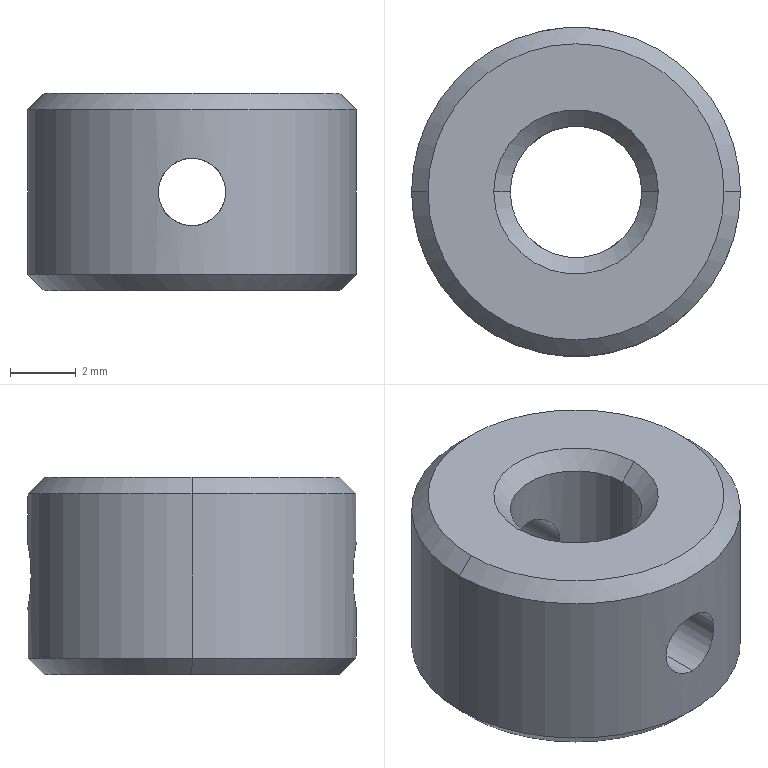Part | SolidWorks | features BaseBody 1, Chamfer 1 | 1 solid | 18 faces | box 10 x 10 x 6 mm | volume 364.767 mm3 | cone 8 | cylinder 8 | plane 2 | commonest cylinder face diameters 2.05 x4 4 x2 10 x2
STEP:
#1=CARTESIAN_POINT('',(-4.5,0.,-3.));
#2=VERTEX_POINT('',#1);
#3=CARTESIAN_POINT('',(4.5,0.,-3.));
#4=VERTEX_POINT('',#3);
#5=CARTESIAN_POINT('',(0.,0.,-3.));
#6=DIRECTION('',(0.,0.,-1.));
#7=DIRECTION('',(1.,0.,0.));
#8=AXIS2_PLACEMENT_3D('',#5,#6,#7);
#9=CIRCLE('',#8,4.5);
#10=EDGE_CURVE('',#2,#4,#9,.T.);
#11=ORIENTED_EDGE('',*,*,#10,.F.);
#12=CARTESIAN_POINT('',(-5.,0.,-2.5));
#13=VERTEX_POINT('',#12);
#14=CARTESIAN_POINT('',(-5.,0.,-2.5));
#15=DIRECTION('',(-0.7071,0.,0.7071));
#16=VECTOR('',#15,1000.);
#17=LINE('',#14,#16);
#18=EDGE_CURVE('',#2,#13,#17,.T.);
#19=ORIENTED_EDGE('',*,*,#18,.T.);
#20=CARTESIAN_POINT('',(5.,0.,-2.5));
#21=VERTEX_POINT('',#20);
#22=CARTESIAN_POINT('',(0.,0.,-2.5));
#23=DIRECTION('',(0.,0.,1.));
#24=DIRECTION('',(1.,0.,0.));
#25=AXIS2_PLACEMENT_3D('',#22,#23,#24);
#26=CIRCLE('',#25,5.);
#27=EDGE_CURVE('',#21,#13,#26,.T.);
#28=ORIENTED_EDGE('',*,*,#27,.F.);
#29=CARTESIAN_POINT('',(5.,0.,-2.5));
#30=DIRECTION('',(0.7071,0.,0.7071));
#31=VECTOR('',#30,1000.);
#32=LINE('',#29,#31);
#33=EDGE_CURVE('',#4,#21,#32,.T.);
#34=ORIENTED_EDGE('',*,*,#33,.F.);
#35=EDGE_LOOP('',(#11,#19,#28,#34));
#36=FACE_OUTER_BOUND('',#35,.T.);
#37=CARTESIAN_POINT('',(0.,0.,-2.5));
#38=DIRECTION('',(0.,0.,1.));
#39=DIRECTION('',(1.,0.,0.));
#40=AXIS2_PLACEMENT_3D('',#37,#38,#39);
#41=CONICAL_SURFACE('',#40,5.,0.7854);
#42=ADVANCED_FACE('',(#36),#41,.T.);
#43=CARTESIAN_POINT('',(4.5,0.,3.));
#44=VERTEX_POINT('',#43);
#45=CARTESIAN_POINT('',(-4.5,0.,3.));
#46=VERTEX_POINT('',#45);
#47=CARTESIAN_POINT('',(0.,0.,3.));
#48=DIRECTION('',(0.,0.,1.));
#49=DIRECTION('',(1.,0.,0.));
#50=AXIS2_PLACEMENT_3D('',#47,#48,#49);
#51=CIRCLE('',#50,4.5);
#52=EDGE_CURVE('',#44,#46,#51,.T.);
#53=ORIENTED_EDGE('',*,*,#52,.F.);
#54=CARTESIAN_POINT('',(5.,0.,2.5));
#55=VERTEX_POINT('',#54);
#56=CARTESIAN_POINT('',(5.,0.,2.5));
#57=DIRECTION('',(0.7071,0.,-0.7071));
#58=VECTOR('',#57,1000.);
#59=LINE('',#56,#58);
#60=EDGE_CURVE('',#44,#55,#59,.T.);
#61=ORIENTED_EDGE('',*,*,#60,.T.);
#62=CARTESIAN_POINT('',(-5.,0.,2.5));
#63=VERTEX_POINT('',#62);
#64=CARTESIAN_POINT('',(0.,0.,2.5));
#65=DIRECTION('',(0.,0.,-1.));
#66=DIRECTION('',(1.,0.,0.));
#67=AXIS2_PLACEMENT_3D('',#64,#65,#66);
#68=CIRCLE('',#67,5.);
#69=EDGE_CURVE('',#63,#55,#68,.T.);
#70=ORIENTED_EDGE('',*,*,#69,.F.);
#71=CARTESIAN_POINT('',(-5.,0.,2.5));
#72=DIRECTION('',(-0.7071,0.,-0.7071));
#73=VECTOR('',#72,1000.);
#74=LINE('',#71,#73);
#75=EDGE_CURVE('',#46,#63,#74,.T.);
#76=ORIENTED_EDGE('',*,*,#75,.F.);
#77=EDGE_LOOP('',(#53,#61,#70,#76));
#78=FACE_OUTER_BOUND('',#77,.T.);
#79=CARTESIAN_POINT('',(0.,0.,2.5));
#80=DIRECTION('',(0.,0.,-1.));
#81=DIRECTION('',(-1.,0.,0.));
#82=AXIS2_PLACEMENT_3D('',#79,#80,#81);
#83=CONICAL_SURFACE('',#82,5.,0.7854);
#84=ADVANCED_FACE('',(#78),#83,.T.);
#85=CARTESIAN_POINT('',(-2.,0.,2.5));
#86=VERTEX_POINT('',#85);
#87=CARTESIAN_POINT('',(2.,0.,2.5));
#88=VERTEX_POINT('',#87);
#89=CARTESIAN_POINT('',(0.,0.,2.5));
#90=DIRECTION('',(0.,0.,1.));
#91=DIRECTION('',(1.,0.,0.));
#92=AXIS2_PLACEMENT_3D('',#89,#90,#91);
#93=CIRCLE('',#92,2.);
#94=EDGE_CURVE('',#86,#88,#93,.T.);
#95=ORIENTED_EDGE('',*,*,#94,.F.);
#96=CARTESIAN_POINT('',(-2.5,0.,3.));
#97=VERTEX_POINT('',#96);
#98=CARTESIAN_POINT('',(-2.5,0.,3.));
#99=DIRECTION('',(-0.7071,0.,0.7071));
#100=VECTOR('',#99,1000.);
#101=LINE('',#98,#100);
#102=EDGE_CURVE('',#86,#97,#101,.T.);
#103=ORIENTED_EDGE('',*,*,#102,.T.);
#104=CARTESIAN_POINT('',(2.5,0.,3.));
#105=VERTEX_POINT('',#104);
#106=CARTESIAN_POINT('',(0.,0.,3.));
#107=DIRECTION('',(0.,0.,-1.));
#108=DIRECTION('',(1.,0.,0.));
#109=AXIS2_PLACEMENT_3D('',#106,#107,#108);
#110=CIRCLE('',#109,2.5);
#111=EDGE_CURVE('',#105,#97,#110,.T.);
#112=ORIENTED_EDGE('',*,*,#111,.F.);
#113=CARTESIAN_POINT('',(2.5,0.,3.));
#114=DIRECTION('',(0.7071,0.,0.7071));
#115=VECTOR('',#114,1000.);
#116=LINE('',#113,#115);
#117=EDGE_CURVE('',#88,#105,#116,.T.);
#118=ORIENTED_EDGE('',*,*,#117,.F.);
#119=EDGE_LOOP('',(#95,#103,#112,#118));
#120=FACE_OUTER_BOUND('',#119,.T.);
#121=CARTESIAN_POINT('',(0.,0.,3.));
#122=DIRECTION('',(0.,0.,1.));
#123=DIRECTION('',(1.,0.,0.));
#124=AXIS2_PLACEMENT_3D('',#121,#122,#123);
#125=CONICAL_SURFACE('',#124,2.5,0.7854);
#126=ADVANCED_FACE('',(#120),#125,.F.);
#127=CARTESIAN_POINT('',(2.,0.,-2.5));
#128=VERTEX_POINT('',#127);
#129=CARTESIAN_POINT('',(-2.,0.,-2.5));
#130=VERTEX_POINT('',#129);
#131=CARTESIAN_POINT('',(0.,0.,-2.5));
#132=DIRECTION('',(0.,0.,-1.));
#133=DIRECTION('',(1.,0.,0.));
#134=AXIS2_PLACEMENT_3D('',#131,#132,#133);
#135=CIRCLE('',#134,2.);
#136=EDGE_CURVE('',#128,#130,#135,.T.);
#137=ORIENTED_EDGE('',*,*,#136,.F.);
#138=CARTESIAN_POINT('',(2.5,0.,-3.));
#139=VERTEX_POINT('',#138);
#140=CARTESIAN_POINT('',(2.,0.,-2.5));
#141=DIRECTION('',(0.7071,0.,-0.7071));
#142=VECTOR('',#141,1000.);
#143=LINE('',#140,#142);
#144=EDGE_CURVE('',#128,#139,#143,.T.);
#145=ORIENTED_EDGE('',*,*,#144,.T.);
#146=CARTESIAN_POINT('',(-2.5,0.,-3.));
#147=VERTEX_POINT('',#146);
#148=CARTESIAN_POINT('',(0.,0.,-3.));
#149=DIRECTION('',(0.,0.,1.));
#150=DIRECTION('',(1.,0.,0.));
#151=AXIS2_PLACEMENT_3D('',#148,#149,#150);
#152=CIRCLE('',#151,2.5);
#153=EDGE_CURVE('',#147,#139,#152,.T.);
#154=ORIENTED_EDGE('',*,*,#153,.F.);
#155=CARTESIAN_POINT('',(-2.,0.,-2.5));
#156=DIRECTION('',(-0.7071,0.,-0.7071));
#157=VECTOR('',#156,1000.);
#158=LINE('',#155,#157);
#159=EDGE_CURVE('',#130,#147,#158,.T.);
#160=ORIENTED_EDGE('',*,*,#159,.F.);
#161=EDGE_LOOP('',(#137,#145,#154,#160));
#162=FACE_OUTER_BOUND('',#161,.T.);
#163=CARTESIAN_POINT('',(0.,0.,-2.5));
#164=DIRECTION('',(0.,0.,-1.));
#165=DIRECTION('',(-1.,0.,0.));
#166=AXIS2_PLACEMENT_3D('',#163,#164,#165);
#167=CONICAL_SURFACE('',#166,2.,0.7854);
#168=ADVANCED_FACE('',(#162),#167,.F.);
#169=CARTESIAN_POINT('',(0.,5.,-1.025));
#170=VERTEX_POINT('',#169);
#171=CARTESIAN_POINT('',(0.,5.,1.025));
#172=VERTEX_POINT('',#171);
#173=CARTESIAN_POINT('',(0.,5.,-1.025));
#174=CARTESIAN_POINT('',(0.1358,5.,-1.025));
#175=CARTESIAN_POINT('',(0.269,4.994,-0.9981));
#176=CARTESIAN_POINT('',(0.5171,4.975,-0.8951));
#177=CARTESIAN_POINT('',(0.6306,4.961,-0.819));
#178=CARTESIAN_POINT('',(0.8191,4.933,-0.6305));
#179=CARTESIAN_POINT('',(0.8954,4.919,-0.5165));
#180=CARTESIAN_POINT('',(0.9978,4.9,-0.27));
#181=CARTESIAN_POINT('',(1.025,4.894,-0.1349));
#182=CARTESIAN_POINT('',(1.025,4.894,0.1332));
#183=CARTESIAN_POINT('',(0.9985,4.9,0.2677));
#184=CARTESIAN_POINT('',(0.8956,4.919,0.5163));
#185=CARTESIAN_POINT('',(0.8204,4.933,0.6291));
#186=CARTESIAN_POINT('',(0.63,4.961,0.8197));
#187=CARTESIAN_POINT('',(0.5172,4.975,0.895));
#188=CARTESIAN_POINT('',(0.2695,4.994,0.998));
#189=CARTESIAN_POINT('',(0.1358,5.,1.025));
#190=CARTESIAN_POINT('',(0.,5.,1.025));
#191=B_SPLINE_CURVE_WITH_KNOTS('',3,(#173,#174,#175,#176,#177,#178,#179,#180,#181,#182,#183,#184,#185,#186,#187,#188,#189,#190),.UNSPECIFIED.,.F.,.F.,(4,2,2,2,2,2,2,2,4),(0.,0.0004015,0.0008031,0.001205,0.001606,0.002008,0.002409,0.002811,0.003212),.UNSPECIFIED.);
#192=EDGE_CURVE('',#170,#172,#191,.T.);
#193=ORIENTED_EDGE('',*,*,#192,.T.);
#194=CARTESIAN_POINT('',(0.,5.,1.025));
#195=CARTESIAN_POINT('',(-0.1358,5.,1.025));
#196=CARTESIAN_POINT('',(-0.269,4.994,0.9981));
#197=CARTESIAN_POINT('',(-0.5171,4.975,0.8951));
#198=CARTESIAN_POINT('',(-0.6306,4.961,0.819));
#199=CARTESIAN_POINT('',(-0.8191,4.933,0.6305));
#200=CARTESIAN_POINT('',(-0.8954,4.919,0.5165));
#201=CARTESIAN_POINT('',(-0.9978,4.9,0.27));
#202=CARTESIAN_POINT('',(-1.025,4.894,0.1349));
#203=CARTESIAN_POINT('',(-1.025,4.894,-0.1332));
#204=CARTESIAN_POINT('',(-0.9985,4.9,-0.2677));
#205=CARTESIAN_POINT('',(-0.8956,4.919,-0.5163));
#206=CARTESIAN_POINT('',(-0.8204,4.933,-0.6291));
#207=CARTESIAN_POINT('',(-0.63,4.961,-0.8197));
#208=CARTESIAN_POINT('',(-0.5172,4.975,-0.895));
#209=CARTESIAN_POINT('',(-0.2695,4.994,-0.998));
#210=CARTESIAN_POINT('',(-0.1358,5.,-1.025));
#211=CARTESIAN_POINT('',(0.,5.,-1.025));
#212=B_SPLINE_CURVE_WITH_KNOTS('',3,(#194,#195,#196,#197,#198,#199,#200,#201,#202,#203,#204,#205,#206,#207,#208,#209,#210,#211),.UNSPECIFIED.,.F.,.F.,(4,2,2,2,2,2,2,2,4),(0.003212,0.003614,0.004015,0.004417,0.004818,0.00522,0.005621,0.006023,0.006425),.UNSPECIFIED.);
#213=EDGE_CURVE('',#172,#170,#212,.T.);
#214=ORIENTED_EDGE('',*,*,#213,.T.);
#215=EDGE_LOOP('',(#193,#214));
#216=FACE_BOUND('',#215,.T.);
#217=ORIENTED_EDGE('',*,*,#69,.T.);
#218=CARTESIAN_POINT('',(5.,0.,3.));
#219=DIRECTION('',(0.,0.,-1.));
#220=VECTOR('',#219,1000.);
#221=LINE('',#218,#220);
#222=EDGE_CURVE('',#55,#21,#221,.T.);
#223=ORIENTED_EDGE('',*,*,#222,.T.);
#224=ORIENTED_EDGE('',*,*,#27,.T.);
#225=CARTESIAN_POINT('',(-5.,0.,3.));
#226=DIRECTION('',(0.,0.,-1.));
#227=VECTOR('',#226,1000.);
#228=LINE('',#225,#227);
#229=EDGE_CURVE('',#63,#13,#228,.T.);
#230=ORIENTED_EDGE('',*,*,#229,.F.);
#231=EDGE_LOOP('',(#217,#223,#224,#230));
#232=FACE_OUTER_BOUND('',#231,.T.);
#233=CARTESIAN_POINT('',(0.,0.,3.));
#234=DIRECTION('',(0.,0.,-1.));
#235=DIRECTION('',(-1.,0.,0.));
#236=AXIS2_PLACEMENT_3D('',#233,#234,#235);
#237=CYLINDRICAL_SURFACE('',#236,5.);
#238=ADVANCED_FACE('',(#216,#232),#237,.T.);
#239=ORIENTED_EDGE('',*,*,#213,.F.);
#240=CARTESIAN_POINT('',(0.,2.,1.025));
#241=VERTEX_POINT('',#240);
#242=CARTESIAN_POINT('',(0.,0.,1.025));
#243=DIRECTION('',(0.,-1.,0.));
#244=VECTOR('',#243,1000.);
#245=LINE('',#242,#244);
#246=EDGE_CURVE('',#172,#241,#245,.T.);
#247=ORIENTED_EDGE('',*,*,#246,.T.);
#248=CARTESIAN_POINT('',(0.,2.,-1.025));
#249=VERTEX_POINT('',#248);
#250=CARTESIAN_POINT('',(0.,2.,-1.025));
#251=CARTESIAN_POINT('',(-0.138,2.,-1.025));
#252=CARTESIAN_POINT('',(-0.2732,1.985,-0.997));
#253=CARTESIAN_POINT('',(-0.5207,1.935,-0.893));
#254=CARTESIAN_POINT('',(-0.6326,1.9,-0.8171));
#255=CARTESIAN_POINT('',(-0.8181,1.828,-0.6313));
#256=CARTESIAN_POINT('',(-0.8935,1.79,-0.5197));
#257=CARTESIAN_POINT('',(-0.9965,1.735,-0.2744));
#258=CARTESIAN_POINT('',(-1.025,1.718,-0.1384));
#259=CARTESIAN_POINT('',(-1.025,1.717,0.1346));
#260=CARTESIAN_POINT('',(-0.9975,1.734,0.2713));
#261=CARTESIAN_POINT('',(-0.8938,1.79,0.5194));
#262=CARTESIAN_POINT('',(-0.8185,1.828,0.6308));
#263=CARTESIAN_POINT('',(-0.633,1.9,0.8168));
#264=CARTESIAN_POINT('',(-0.5207,1.935,0.8929));
#265=CARTESIAN_POINT('',(-0.2749,1.985,0.9964));
#266=CARTESIAN_POINT('',(-0.1382,2.,1.025));
#267=CARTESIAN_POINT('',(0.,2.,1.025));
#268=B_SPLINE_CURVE_WITH_KNOTS('',3,(#250,#251,#252,#253,#254,#255,#256,#257,#258,#259,#260,#261,#262,#263,#264,#265,#266,#267),.UNSPECIFIED.,.F.,.F.,(4,2,2,2,2,2,2,2,4),(0.,0.0004078,0.0008155,0.001223,0.001631,0.002039,0.002447,0.002854,0.003262),.UNSPECIFIED.);
#269=EDGE_CURVE('',#249,#241,#268,.T.);
#270=ORIENTED_EDGE('',*,*,#269,.F.);
#271=CARTESIAN_POINT('',(0.,0.,-1.025));
#272=DIRECTION('',(0.,-1.,0.));
#273=VECTOR('',#272,1000.);
#274=LINE('',#271,#273);
#275=EDGE_CURVE('',#170,#249,#274,.T.);
#276=ORIENTED_EDGE('',*,*,#275,.F.);
#277=EDGE_LOOP('',(#239,#247,#270,#276));
#278=FACE_OUTER_BOUND('',#277,.T.);
#279=CARTESIAN_POINT('',(0.,0.,0.));
#280=DIRECTION('',(0.,-1.,0.));
#281=DIRECTION('',(0.,0.,-1.));
#282=AXIS2_PLACEMENT_3D('',#279,#280,#281);
#283=CYLINDRICAL_SURFACE('',#282,1.025);
#284=ADVANCED_FACE('',(#278),#283,.F.);
#285=CARTESIAN_POINT('',(0.,-5.,-1.025));
#286=VERTEX_POINT('',#285);
#287=CARTESIAN_POINT('',(0.,-5.,1.025));
#288=VERTEX_POINT('',#287);
#289=CARTESIAN_POINT('',(0.,-5.,-1.025));
#290=CARTESIAN_POINT('',(-0.1358,-5.,-1.025));
#291=CARTESIAN_POINT('',(-0.269,-4.994,-0.9981));
#292=CARTESIAN_POINT('',(-0.5171,-4.975,-0.8951));
#293=CARTESIAN_POINT('',(-0.6306,-4.961,-0.819));
#294=CARTESIAN_POINT('',(-0.8191,-4.933,-0.6305));
#295=CARTESIAN_POINT('',(-0.8954,-4.919,-0.5165));
#296=CARTESIAN_POINT('',(-0.9978,-4.9,-0.27));
#297=CARTESIAN_POINT('',(-1.025,-4.894,-0.1349));
#298=CARTESIAN_POINT('',(-1.025,-4.894,0.1332));
#299=CARTESIAN_POINT('',(-0.9985,-4.9,0.2677));
#300=CARTESIAN_POINT('',(-0.8956,-4.919,0.5163));
#301=CARTESIAN_POINT('',(-0.8204,-4.933,0.6291));
#302=CARTESIAN_POINT('',(-0.63,-4.961,0.8197));
#303=CARTESIAN_POINT('',(-0.5172,-4.975,0.895));
#304=CARTESIAN_POINT('',(-0.2695,-4.994,0.998));
#305=CARTESIAN_POINT('',(-0.1358,-5.,1.025));
#306=CARTESIAN_POINT('',(0.,-5.,1.025));
#307=B_SPLINE_CURVE_WITH_KNOTS('',3,(#289,#290,#291,#292,#293,#294,#295,#296,#297,#298,#299,#300,#301,#302,#303,#304,#305,#306),.UNSPECIFIED.,.F.,.F.,(4,2,2,2,2,2,2,2,4),(0.,0.0004015,0.0008031,0.001205,0.001606,0.002008,0.002409,0.002811,0.003212),.UNSPECIFIED.);
#308=EDGE_CURVE('',#286,#288,#307,.T.);
#309=ORIENTED_EDGE('',*,*,#308,.F.);
#310=CARTESIAN_POINT('',(0.,-2.,-1.025));
#311=VERTEX_POINT('',#310);
#312=CARTESIAN_POINT('',(0.,0.,-1.025));
#313=DIRECTION('',(0.,1.,0.));
#314=VECTOR('',#313,1000.);
#315=LINE('',#312,#314);
#316=EDGE_CURVE('',#286,#311,#315,.T.);
#317=ORIENTED_EDGE('',*,*,#316,.T.);
#318=CARTESIAN_POINT('',(0.,-2.,1.025));
#319=VERTEX_POINT('',#318);
#320=CARTESIAN_POINT('',(0.,-2.,1.025));
#321=CARTESIAN_POINT('',(-0.138,-2.,1.025));
#322=CARTESIAN_POINT('',(-0.2732,-1.985,0.997));
#323=CARTESIAN_POINT('',(-0.5207,-1.935,0.893));
#324=CARTESIAN_POINT('',(-0.6326,-1.9,0.8171));
#325=CARTESIAN_POINT('',(-0.8181,-1.828,0.6313));
#326=CARTESIAN_POINT('',(-0.8935,-1.79,0.5197));
#327=CARTESIAN_POINT('',(-0.9965,-1.735,0.2744));
#328=CARTESIAN_POINT('',(-1.025,-1.718,0.1384));
#329=CARTESIAN_POINT('',(-1.025,-1.717,-0.1346));
#330=CARTESIAN_POINT('',(-0.9975,-1.734,-0.2713));
#331=CARTESIAN_POINT('',(-0.8938,-1.79,-0.5194));
#332=CARTESIAN_POINT('',(-0.8185,-1.828,-0.6308));
#333=CARTESIAN_POINT('',(-0.633,-1.9,-0.8168));
#334=CARTESIAN_POINT('',(-0.5207,-1.935,-0.8929));
#335=CARTESIAN_POINT('',(-0.2749,-1.985,-0.9964));
#336=CARTESIAN_POINT('',(-0.1382,-2.,-1.025));
#337=CARTESIAN_POINT('',(0.,-2.,-1.025));
#338=B_SPLINE_CURVE_WITH_KNOTS('',3,(#320,#321,#322,#323,#324,#325,#326,#327,#328,#329,#330,#331,#332,#333,#334,#335,#336,#337),.UNSPECIFIED.,.F.,.F.,(4,2,2,2,2,2,2,2,4),(0.,0.0004078,0.0008155,0.001223,0.001631,0.002039,0.002447,0.002854,0.003262),.UNSPECIFIED.);
#339=EDGE_CURVE('',#319,#311,#338,.T.);
#340=ORIENTED_EDGE('',*,*,#339,.F.);
#341=CARTESIAN_POINT('',(0.,0.,1.025));
#342=DIRECTION('',(0.,1.,0.));
#343=VECTOR('',#342,1000.);
#344=LINE('',#341,#343);
#345=EDGE_CURVE('',#288,#319,#344,.T.);
#346=ORIENTED_EDGE('',*,*,#345,.F.);
#347=EDGE_LOOP('',(#309,#317,#340,#346));
#348=FACE_OUTER_BOUND('',#347,.T.);
#349=CARTESIAN_POINT('',(0.,0.,0.));
#350=DIRECTION('',(0.,1.,0.));
#351=DIRECTION('',(0.,0.,1.));
#352=AXIS2_PLACEMENT_3D('',#349,#350,#351);
#353=CYLINDRICAL_SURFACE('',#352,1.025);
#354=ADVANCED_FACE('',(#348),#353,.F.);
#355=ORIENTED_EDGE('',*,*,#339,.T.);
#356=CARTESIAN_POINT('',(0.,-2.,-1.025));
#357=CARTESIAN_POINT('',(0.138,-2.,-1.025));
#358=CARTESIAN_POINT('',(0.2732,-1.985,-0.997));
#359=CARTESIAN_POINT('',(0.5207,-1.935,-0.893));
#360=CARTESIAN_POINT('',(0.6326,-1.9,-0.8171));
#361=CARTESIAN_POINT('',(0.8181,-1.828,-0.6313));
#362=CARTESIAN_POINT('',(0.8935,-1.79,-0.5197));
#363=CARTESIAN_POINT('',(0.9965,-1.735,-0.2744));
#364=CARTESIAN_POINT('',(1.025,-1.718,-0.1384));
#365=CARTESIAN_POINT('',(1.025,-1.717,0.1346));
#366=CARTESIAN_POINT('',(0.9975,-1.734,0.2713));
#367=CARTESIAN_POINT('',(0.8938,-1.79,0.5194));
#368=CARTESIAN_POINT('',(0.8185,-1.828,0.6308));
#369=CARTESIAN_POINT('',(0.633,-1.9,0.8168));
#370=CARTESIAN_POINT('',(0.5207,-1.935,0.8929));
#371=CARTESIAN_POINT('',(0.2749,-1.985,0.9964));
#372=CARTESIAN_POINT('',(0.1379,-2.,1.025));
#373=CARTESIAN_POINT('',(0.,-2.,1.025));
#374=B_SPLINE_CURVE_WITH_KNOTS('',3,(#356,#357,#358,#359,#360,#361,#362,#363,#364,#365,#366,#367,#368,#369,#370,#371,#372,#373),.UNSPECIFIED.,.F.,.F.,(4,2,2,2,2,2,2,2,4),(0.003262,0.003669,0.004077,0.004484,0.004891,0.005299,0.005706,0.006114,0.006521),.UNSPECIFIED.);
#375=EDGE_CURVE('',#311,#319,#374,.T.);
#376=ORIENTED_EDGE('',*,*,#375,.T.);
#377=EDGE_LOOP('',(#355,#376));
#378=FACE_BOUND('',#377,.T.);
#379=ORIENTED_EDGE('',*,*,#94,.T.);
#380=CARTESIAN_POINT('',(2.,0.,3.));
#381=DIRECTION('',(0.,0.,-1.));
#382=VECTOR('',#381,1000.);
#383=LINE('',#380,#382);
#384=EDGE_CURVE('',#88,#128,#383,.T.);
#385=ORIENTED_EDGE('',*,*,#384,.T.);
#386=ORIENTED_EDGE('',*,*,#136,.T.);
#387=CARTESIAN_POINT('',(-2.,0.,3.));
#388=DIRECTION('',(0.,0.,-1.));
#389=VECTOR('',#388,1000.);
#390=LINE('',#387,#389);
#391=EDGE_CURVE('',#86,#130,#390,.T.);
#392=ORIENTED_EDGE('',*,*,#391,.F.);
#393=EDGE_LOOP('',(#379,#385,#386,#392));
#394=FACE_OUTER_BOUND('',#393,.T.);
#395=CARTESIAN_POINT('',(0.,0.,3.));
#396=DIRECTION('',(0.,0.,-1.));
#397=DIRECTION('',(-1.,0.,0.));
#398=AXIS2_PLACEMENT_3D('',#395,#396,#397);
#399=CYLINDRICAL_SURFACE('',#398,2.);
#400=ADVANCED_FACE('',(#378,#394),#399,.F.);
#401=ORIENTED_EDGE('',*,*,#222,.F.);
#402=CARTESIAN_POINT('',(0.,0.,2.5));
#403=DIRECTION('',(0.,0.,-1.));
#404=DIRECTION('',(1.,0.,0.));
#405=AXIS2_PLACEMENT_3D('',#402,#403,#404);
#406=CIRCLE('',#405,5.);
#407=EDGE_CURVE('',#55,#63,#406,.T.);
#408=ORIENTED_EDGE('',*,*,#407,.T.);
#409=ORIENTED_EDGE('',*,*,#229,.T.);
#410=CARTESIAN_POINT('',(0.,0.,-2.5));
#411=DIRECTION('',(0.,0.,1.));
#412=DIRECTION('',(1.,0.,0.));
#413=AXIS2_PLACEMENT_3D('',#410,#411,#412);
#414=CIRCLE('',#413,5.);
#415=EDGE_CURVE('',#13,#21,#414,.T.);
#416=ORIENTED_EDGE('',*,*,#415,.T.);
#417=EDGE_LOOP('',(#401,#408,#409,#416));
#418=FACE_OUTER_BOUND('',#417,.T.);
#419=CARTESIAN_POINT('',(0.,-5.,1.025));
#420=CARTESIAN_POINT('',(0.1358,-5.,1.025));
#421=CARTESIAN_POINT('',(0.269,-4.994,0.9981));
#422=CARTESIAN_POINT('',(0.5171,-4.975,0.8951));
#423=CARTESIAN_POINT('',(0.6306,-4.961,0.819));
#424=CARTESIAN_POINT('',(0.8191,-4.933,0.6305));
#425=CARTESIAN_POINT('',(0.8954,-4.919,0.5165));
#426=CARTESIAN_POINT('',(0.9978,-4.9,0.27));
#427=CARTESIAN_POINT('',(1.025,-4.894,0.1349));
#428=CARTESIAN_POINT('',(1.025,-4.894,-0.1332));
#429=CARTESIAN_POINT('',(0.9985,-4.9,-0.2677));
#430=CARTESIAN_POINT('',(0.8956,-4.919,-0.5163));
#431=CARTESIAN_POINT('',(0.8204,-4.933,-0.6291));
#432=CARTESIAN_POINT('',(0.63,-4.961,-0.8197));
#433=CARTESIAN_POINT('',(0.5172,-4.975,-0.895));
#434=CARTESIAN_POINT('',(0.2695,-4.994,-0.998));
#435=CARTESIAN_POINT('',(0.1358,-5.,-1.025));
#436=CARTESIAN_POINT('',(0.,-5.,-1.025));
#437=B_SPLINE_CURVE_WITH_KNOTS('',3,(#419,#420,#421,#422,#423,#424,#425,#426,#427,#428,#429,#430,#431,#432,#433,#434,#435,#436),.UNSPECIFIED.,.F.,.F.,(4,2,2,2,2,2,2,2,4),(0.003212,0.003614,0.004015,0.004417,0.004818,0.00522,0.005621,0.006023,0.006425),.UNSPECIFIED.);
#438=EDGE_CURVE('',#288,#286,#437,.T.);
#439=ORIENTED_EDGE('',*,*,#438,.T.);
#440=ORIENTED_EDGE('',*,*,#308,.T.);
#441=EDGE_LOOP('',(#439,#440));
#442=FACE_BOUND('',#441,.T.);
#443=CARTESIAN_POINT('',(0.,0.,3.));
#444=DIRECTION('',(0.,0.,-1.));
#445=DIRECTION('',(-1.,0.,0.));
#446=AXIS2_PLACEMENT_3D('',#443,#444,#445);
#447=CYLINDRICAL_SURFACE('',#446,5.);
#448=ADVANCED_FACE('',(#418,#442),#447,.T.);
#449=ORIENTED_EDGE('',*,*,#153,.T.);
#450=CARTESIAN_POINT('',(0.,0.,-3.));
#451=DIRECTION('',(0.,0.,1.));
#452=DIRECTION('',(1.,0.,0.));
#453=AXIS2_PLACEMENT_3D('',#450,#451,#452);
#454=CIRCLE('',#453,2.5);
#455=EDGE_CURVE('',#139,#147,#454,.T.);
#456=ORIENTED_EDGE('',*,*,#455,.T.);
#457=EDGE_LOOP('',(#449,#456));
#458=FACE_BOUND('',#457,.T.);
#459=CARTESIAN_POINT('',(0.,0.,-3.));
#460=DIRECTION('',(0.,0.,-1.));
#461=DIRECTION('',(1.,0.,0.));
#462=AXIS2_PLACEMENT_3D('',#459,#460,#461);
#463=CIRCLE('',#462,4.5);
#464=EDGE_CURVE('',#4,#2,#463,.T.);
#465=ORIENTED_EDGE('',*,*,#464,.T.);
#466=ORIENTED_EDGE('',*,*,#10,.T.);
#467=EDGE_LOOP('',(#465,#466));
#468=FACE_OUTER_BOUND('',#467,.T.);
#469=CARTESIAN_POINT('',(0.,0.,-3.));
#470=DIRECTION('',(0.,0.,1.));
#471=DIRECTION('',(1.,0.,0.));
#472=AXIS2_PLACEMENT_3D('',#469,#470,#471);
#473=PLANE('',#472);
#474=ADVANCED_FACE('',(#458,#468),#473,.F.);
#475=ORIENTED_EDGE('',*,*,#111,.T.);
#476=CARTESIAN_POINT('',(0.,0.,3.));
#477=DIRECTION('',(0.,0.,-1.));
#478=DIRECTION('',(1.,0.,0.));
#479=AXIS2_PLACEMENT_3D('',#476,#477,#478);
#480=CIRCLE('',#479,2.5);
#481=EDGE_CURVE('',#97,#105,#480,.T.);
#482=ORIENTED_EDGE('',*,*,#481,.T.);
#483=EDGE_LOOP('',(#475,#482));
#484=FACE_BOUND('',#483,.T.);
#485=CARTESIAN_POINT('',(0.,0.,3.));
#486=DIRECTION('',(0.,0.,1.));
#487=DIRECTION('',(1.,0.,0.));
#488=AXIS2_PLACEMENT_3D('',#485,#486,#487);
#489=CIRCLE('',#488,4.5);
#490=EDGE_CURVE('',#46,#44,#489,.T.);
#491=ORIENTED_EDGE('',*,*,#490,.T.);
#492=ORIENTED_EDGE('',*,*,#52,.T.);
#493=EDGE_LOOP('',(#491,#492));
#494=FACE_OUTER_BOUND('',#493,.T.);
#495=CARTESIAN_POINT('',(0.,0.,3.));
#496=DIRECTION('',(0.,0.,1.));
#497=DIRECTION('',(1.,0.,0.));
#498=AXIS2_PLACEMENT_3D('',#495,#496,#497);
#499=PLANE('',#498);
#500=ADVANCED_FACE('',(#484,#494),#499,.T.);
#501=ORIENTED_EDGE('',*,*,#246,.F.);
#502=ORIENTED_EDGE('',*,*,#192,.F.);
#503=ORIENTED_EDGE('',*,*,#275,.T.);
#504=CARTESIAN_POINT('',(0.,2.,1.025));
#505=CARTESIAN_POINT('',(0.138,2.,1.025));
#506=CARTESIAN_POINT('',(0.2732,1.985,0.997));
#507=CARTESIAN_POINT('',(0.5207,1.935,0.893));
#508=CARTESIAN_POINT('',(0.6326,1.9,0.8171));
#509=CARTESIAN_POINT('',(0.8181,1.828,0.6313));
#510=CARTESIAN_POINT('',(0.8935,1.79,0.5197));
#511=CARTESIAN_POINT('',(0.9965,1.735,0.2744));
#512=CARTESIAN_POINT('',(1.025,1.718,0.1384));
#513=CARTESIAN_POINT('',(1.025,1.717,-0.1346));
#514=CARTESIAN_POINT('',(0.9975,1.734,-0.2713));
#515=CARTESIAN_POINT('',(0.8938,1.79,-0.5194));
#516=CARTESIAN_POINT('',(0.8185,1.828,-0.6308));
#517=CARTESIAN_POINT('',(0.633,1.9,-0.8168));
#518=CARTESIAN_POINT('',(0.5207,1.935,-0.8929));
#519=CARTESIAN_POINT('',(0.2749,1.985,-0.9964));
#520=CARTESIAN_POINT('',(0.1379,2.,-1.025));
#521=CARTESIAN_POINT('',(0.,2.,-1.025));
#522=B_SPLINE_CURVE_WITH_KNOTS('',3,(#504,#505,#506,#507,#508,#509,#510,#511,#512,#513,#514,#515,#516,#517,#518,#519,#520,#521),.UNSPECIFIED.,.F.,.F.,(4,2,2,2,2,2,2,2,4),(0.003262,0.003669,0.004077,0.004484,0.004891,0.005299,0.005706,0.006114,0.006521),.UNSPECIFIED.);
#523=EDGE_CURVE('',#241,#249,#522,.T.);
#524=ORIENTED_EDGE('',*,*,#523,.F.);
#525=EDGE_LOOP('',(#501,#502,#503,#524));
#526=FACE_OUTER_BOUND('',#525,.T.);
#527=CARTESIAN_POINT('',(0.,0.,0.));
#528=DIRECTION('',(0.,-1.,0.));
#529=DIRECTION('',(0.,0.,-1.));
#530=AXIS2_PLACEMENT_3D('',#527,#528,#529);
#531=CYLINDRICAL_SURFACE('',#530,1.025);
#532=ADVANCED_FACE('',(#526),#531,.F.);
#533=ORIENTED_EDGE('',*,*,#316,.F.);
#534=ORIENTED_EDGE('',*,*,#438,.F.);
#535=ORIENTED_EDGE('',*,*,#345,.T.);
#536=ORIENTED_EDGE('',*,*,#375,.F.);
#537=EDGE_LOOP('',(#533,#534,#535,#536));
#538=FACE_OUTER_BOUND('',#537,.T.);
#539=CARTESIAN_POINT('',(0.,0.,0.));
#540=DIRECTION('',(0.,1.,0.));
#541=DIRECTION('',(0.,0.,1.));
#542=AXIS2_PLACEMENT_3D('',#539,#540,#541);
#543=CYLINDRICAL_SURFACE('',#542,1.025);
#544=ADVANCED_FACE('',(#538),#543,.F.);
#545=ORIENTED_EDGE('',*,*,#384,.F.);
#546=CARTESIAN_POINT('',(0.,0.,2.5));
#547=DIRECTION('',(0.,0.,1.));
#548=DIRECTION('',(1.,0.,0.));
#549=AXIS2_PLACEMENT_3D('',#546,#547,#548);
#550=CIRCLE('',#549,2.);
#551=EDGE_CURVE('',#88,#86,#550,.T.);
#552=ORIENTED_EDGE('',*,*,#551,.T.);
#553=ORIENTED_EDGE('',*,*,#391,.T.);
#554=CARTESIAN_POINT('',(0.,0.,-2.5));
#555=DIRECTION('',(0.,0.,-1.));
#556=DIRECTION('',(1.,0.,0.));
#557=AXIS2_PLACEMENT_3D('',#554,#555,#556);
#558=CIRCLE('',#557,2.);
#559=EDGE_CURVE('',#130,#128,#558,.T.);
#560=ORIENTED_EDGE('',*,*,#559,.T.);
#561=EDGE_LOOP('',(#545,#552,#553,#560));
#562=FACE_OUTER_BOUND('',#561,.T.);
#563=ORIENTED_EDGE('',*,*,#269,.T.);
#564=ORIENTED_EDGE('',*,*,#523,.T.);
#565=EDGE_LOOP('',(#563,#564));
#566=FACE_BOUND('',#565,.T.);
#567=CARTESIAN_POINT('',(0.,0.,3.));
#568=DIRECTION('',(0.,0.,-1.));
#569=DIRECTION('',(-1.,0.,0.));
#570=AXIS2_PLACEMENT_3D('',#567,#568,#569);
#571=CYLINDRICAL_SURFACE('',#570,2.);
#572=ADVANCED_FACE('',(#562,#566),#571,.F.);
#573=ORIENTED_EDGE('',*,*,#144,.F.);
#574=ORIENTED_EDGE('',*,*,#559,.F.);
#575=ORIENTED_EDGE('',*,*,#159,.T.);
#576=ORIENTED_EDGE('',*,*,#455,.F.);
#577=EDGE_LOOP('',(#573,#574,#575,#576));
#578=FACE_OUTER_BOUND('',#577,.T.);
#579=CARTESIAN_POINT('',(0.,0.,-2.5));
#580=DIRECTION('',(0.,0.,-1.));
#581=DIRECTION('',(-1.,0.,0.));
#582=AXIS2_PLACEMENT_3D('',#579,#580,#581);
#583=CONICAL_SURFACE('',#582,2.,0.7854);
#584=ADVANCED_FACE('',(#578),#583,.F.);
#585=ORIENTED_EDGE('',*,*,#102,.F.);
#586=ORIENTED_EDGE('',*,*,#551,.F.);
#587=ORIENTED_EDGE('',*,*,#117,.T.);
#588=ORIENTED_EDGE('',*,*,#481,.F.);
#589=EDGE_LOOP('',(#585,#586,#587,#588));
#590=FACE_OUTER_BOUND('',#589,.T.);
#591=CARTESIAN_POINT('',(0.,0.,3.));
#592=DIRECTION('',(0.,0.,1.));
#593=DIRECTION('',(1.,0.,0.));
#594=AXIS2_PLACEMENT_3D('',#591,#592,#593);
#595=CONICAL_SURFACE('',#594,2.5,0.7854);
#596=ADVANCED_FACE('',(#590),#595,.F.);
#597=ORIENTED_EDGE('',*,*,#60,.F.);
#598=ORIENTED_EDGE('',*,*,#490,.F.);
#599=ORIENTED_EDGE('',*,*,#75,.T.);
#600=ORIENTED_EDGE('',*,*,#407,.F.);
#601=EDGE_LOOP('',(#597,#598,#599,#600));
#602=FACE_OUTER_BOUND('',#601,.T.);
#603=CARTESIAN_POINT('',(0.,0.,2.5));
#604=DIRECTION('',(0.,0.,-1.));
#605=DIRECTION('',(-1.,0.,0.));
#606=AXIS2_PLACEMENT_3D('',#603,#604,#605);
#607=CONICAL_SURFACE('',#606,5.,0.7854);
#608=ADVANCED_FACE('',(#602),#607,.T.);
#609=ORIENTED_EDGE('',*,*,#18,.F.);
#610=ORIENTED_EDGE('',*,*,#464,.F.);
#611=ORIENTED_EDGE('',*,*,#33,.T.);
#612=ORIENTED_EDGE('',*,*,#415,.F.);
#613=EDGE_LOOP('',(#609,#610,#611,#612));
#614=FACE_OUTER_BOUND('',#613,.T.);
#615=CARTESIAN_POINT('',(0.,0.,-2.5));
#616=DIRECTION('',(0.,0.,1.));
#617=DIRECTION('',(1.,0.,0.));
#618=AXIS2_PLACEMENT_3D('',#615,#616,#617);
#619=CONICAL_SURFACE('',#618,5.,0.7854);
#620=ADVANCED_FACE('',(#614),#619,.T.);
#621=CLOSED_SHELL('',(#42,#84,#126,#168,#238,#284,#354,#400,#448,#474,#500,#532,#544,#572,#584,#596,#608,#620));
#622=MANIFOLD_SOLID_BREP('',#621);
#623=CARTESIAN_POINT('',(0.,0.,0.));
#624=DIRECTION('',(0.,0.,1.));
#625=DIRECTION('',(1.,0.,0.));
#626=AXIS2_PLACEMENT_3D('',#623,#624,#625);
#627=(LENGTH_UNIT()NAMED_UNIT(*)SI_UNIT(.MILLI.,.METRE.));
#628=UNCERTAINTY_MEASURE_WITH_UNIT(LENGTH_MEASURE(0.00001),#627,'','');
#629=(NAMED_UNIT(*)PLANE_ANGLE_UNIT()SI_UNIT($,.RADIAN.));
#630=(NAMED_UNIT(*)SI_UNIT($,.STERADIAN.)SOLID_ANGLE_UNIT());
#631=(GEOMETRIC_REPRESENTATION_CONTEXT(3)GLOBAL_UNCERTAINTY_ASSIGNED_CONTEXT((#628))GLOBAL_UNIT_ASSIGNED_CONTEXT((#627,#629,#630))REPRESENTATION_CONTEXT('',''));
#632=ADVANCED_BREP_SHAPE_REPRESENTATION('',(#622,#626),#631);